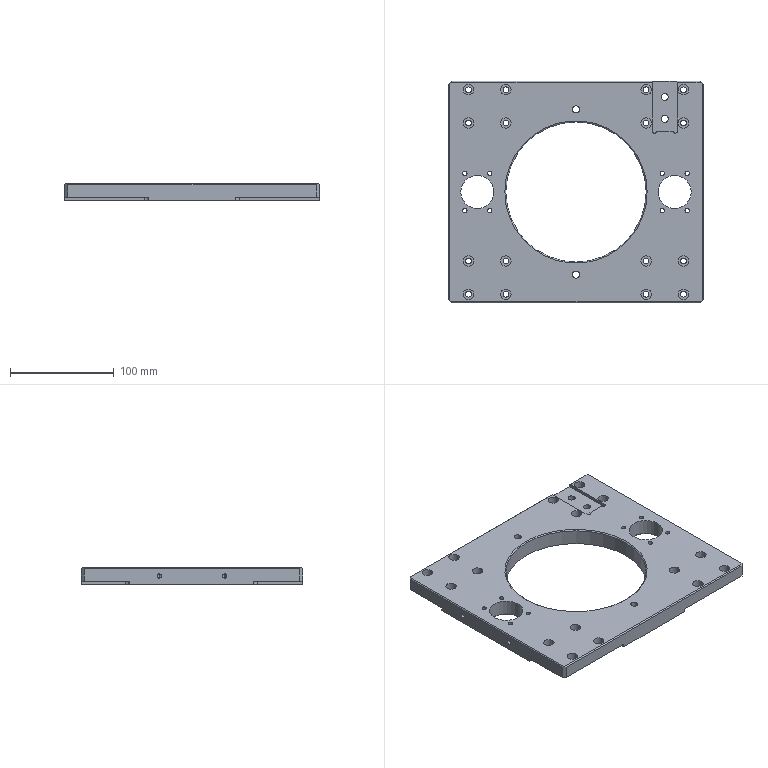Part | SolidWorks | features HoleWzd 7, Chamfer 4, ICE 3, Cut 2, Extrusion 1, Fillet 1 | 1 solid | 185 faces | box 245 x 213 x 16 mm | volume 513654 mm3 | cylinder 116 | plane 47 | cone 22 | commonest cylinder face diameters 5.5 x32 10 x32 4.2 x24 5 x8 6.8 x8 8 x4